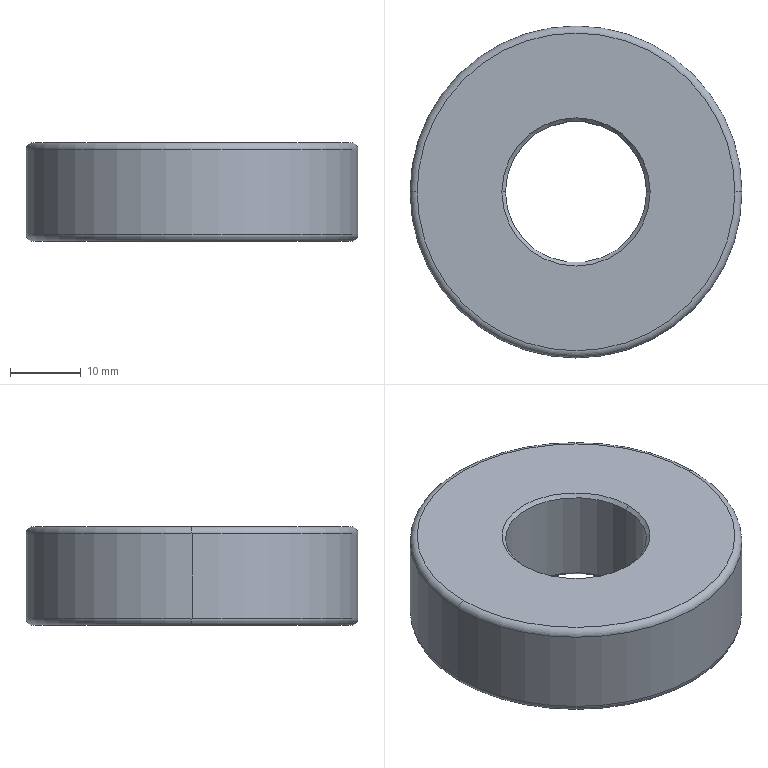Part | SolidWorks | features BaseBody 1 | 1 solid | 14 faces | box 47 x 47 x 14 mm | volume 19812 mm3 | cone 4 | torus 4 | cylinder 4 | plane 2 | commonest cylinder face diameters 20 x2 47 x2
STEP:
#1=CARTESIAN_POINT('',(-10.,0.,13.5));
#2=VERTEX_POINT('',#1);
#3=CARTESIAN_POINT('',(10.,0.,13.5));
#4=VERTEX_POINT('',#3);
#5=CARTESIAN_POINT('',(0.,0.,13.5));
#6=DIRECTION('',(0.,0.,1.));
#7=DIRECTION('',(1.,0.,0.));
#8=AXIS2_PLACEMENT_3D('',#5,#6,#7);
#9=CIRCLE('',#8,10.);
#10=EDGE_CURVE('',#2,#4,#9,.T.);
#11=ORIENTED_EDGE('',*,*,#10,.F.);
#12=CARTESIAN_POINT('',(-10.5,0.,14.));
#13=VERTEX_POINT('',#12);
#14=CARTESIAN_POINT('',(-10.,0.,13.5));
#15=DIRECTION('',(-0.7071,0.,0.7071));
#16=VECTOR('',#15,1000.);
#17=LINE('',#14,#16);
#18=EDGE_CURVE('',#2,#13,#17,.T.);
#19=ORIENTED_EDGE('',*,*,#18,.T.);
#20=CARTESIAN_POINT('',(10.5,0.,14.));
#21=VERTEX_POINT('',#20);
#22=CARTESIAN_POINT('',(0.,0.,14.));
#23=DIRECTION('',(0.,0.,-1.));
#24=DIRECTION('',(1.,0.,0.));
#25=AXIS2_PLACEMENT_3D('',#22,#23,#24);
#26=CIRCLE('',#25,10.5);
#27=EDGE_CURVE('',#21,#13,#26,.T.);
#28=ORIENTED_EDGE('',*,*,#27,.F.);
#29=CARTESIAN_POINT('',(10.,0.,13.5));
#30=DIRECTION('',(0.7071,0.,0.7071));
#31=VECTOR('',#30,1000.);
#32=LINE('',#29,#31);
#33=EDGE_CURVE('',#4,#21,#32,.T.);
#34=ORIENTED_EDGE('',*,*,#33,.F.);
#35=EDGE_LOOP('',(#11,#19,#28,#34));
#36=FACE_OUTER_BOUND('',#35,.T.);
#37=CARTESIAN_POINT('',(0.,0.,13.5));
#38=DIRECTION('',(0.,0.,1.));
#39=DIRECTION('',(1.,0.,0.));
#40=AXIS2_PLACEMENT_3D('',#37,#38,#39);
#41=CONICAL_SURFACE('',#40,10.,0.7854);
#42=ADVANCED_FACE('',(#36),#41,.F.);
#43=CARTESIAN_POINT('',(10.,0.,0.5));
#44=VERTEX_POINT('',#43);
#45=CARTESIAN_POINT('',(-10.,0.,0.5));
#46=VERTEX_POINT('',#45);
#47=CARTESIAN_POINT('',(0.,0.,0.5));
#48=DIRECTION('',(0.,0.,-1.));
#49=DIRECTION('',(1.,0.,0.));
#50=AXIS2_PLACEMENT_3D('',#47,#48,#49);
#51=CIRCLE('',#50,10.);
#52=EDGE_CURVE('',#44,#46,#51,.T.);
#53=ORIENTED_EDGE('',*,*,#52,.F.);
#54=CARTESIAN_POINT('',(10.5,0.,0.));
#55=VERTEX_POINT('',#54);
#56=CARTESIAN_POINT('',(10.5,0.,0.));
#57=DIRECTION('',(0.7071,0.,-0.7071));
#58=VECTOR('',#57,1000.);
#59=LINE('',#56,#58);
#60=EDGE_CURVE('',#44,#55,#59,.T.);
#61=ORIENTED_EDGE('',*,*,#60,.T.);
#62=CARTESIAN_POINT('',(-10.5,0.,0.));
#63=VERTEX_POINT('',#62);
#64=CARTESIAN_POINT('',(0.,0.,0.));
#65=DIRECTION('',(0.,0.,1.));
#66=DIRECTION('',(1.,0.,0.));
#67=AXIS2_PLACEMENT_3D('',#64,#65,#66);
#68=CIRCLE('',#67,10.5);
#69=EDGE_CURVE('',#63,#55,#68,.T.);
#70=ORIENTED_EDGE('',*,*,#69,.F.);
#71=CARTESIAN_POINT('',(-10.5,0.,0.));
#72=DIRECTION('',(-0.7071,0.,-0.7071));
#73=VECTOR('',#72,1000.);
#74=LINE('',#71,#73);
#75=EDGE_CURVE('',#46,#63,#74,.T.);
#76=ORIENTED_EDGE('',*,*,#75,.F.);
#77=EDGE_LOOP('',(#53,#61,#70,#76));
#78=FACE_OUTER_BOUND('',#77,.T.);
#79=CARTESIAN_POINT('',(0.,0.,0.));
#80=DIRECTION('',(0.,0.,-1.));
#81=DIRECTION('',(-1.,0.,0.));
#82=AXIS2_PLACEMENT_3D('',#79,#80,#81);
#83=CONICAL_SURFACE('',#82,10.5,0.7854);
#84=ADVANCED_FACE('',(#78),#83,.F.);
#85=CARTESIAN_POINT('',(-23.5,0.,13.));
#86=VERTEX_POINT('',#85);
#87=CARTESIAN_POINT('',(23.5,0.,13.));
#88=VERTEX_POINT('',#87);
#89=CARTESIAN_POINT('',(0.,0.,13.));
#90=DIRECTION('',(0.,0.,-1.));
#91=DIRECTION('',(1.,0.,0.));
#92=AXIS2_PLACEMENT_3D('',#89,#90,#91);
#93=CIRCLE('',#92,23.5);
#94=EDGE_CURVE('',#86,#88,#93,.T.);
#95=ORIENTED_EDGE('',*,*,#94,.F.);
#96=CARTESIAN_POINT('',(-22.5,0.,14.));
#97=VERTEX_POINT('',#96);
#98=CARTESIAN_POINT('',(-22.5,0.,13.));
#99=DIRECTION('',(0.,1.,0.));
#100=DIRECTION('',(-1.,0.,0.));
#101=AXIS2_PLACEMENT_3D('',#98,#99,#100);
#102=CIRCLE('',#101,1.);
#103=EDGE_CURVE('',#86,#97,#102,.T.);
#104=ORIENTED_EDGE('',*,*,#103,.T.);
#105=CARTESIAN_POINT('',(22.5,0.,14.));
#106=VERTEX_POINT('',#105);
#107=CARTESIAN_POINT('',(0.,0.,14.));
#108=DIRECTION('',(0.,0.,1.));
#109=DIRECTION('',(1.,0.,0.));
#110=AXIS2_PLACEMENT_3D('',#107,#108,#109);
#111=CIRCLE('',#110,22.5);
#112=EDGE_CURVE('',#106,#97,#111,.T.);
#113=ORIENTED_EDGE('',*,*,#112,.F.);
#114=CARTESIAN_POINT('',(22.5,0.,13.));
#115=DIRECTION('',(0.,-1.,0.));
#116=DIRECTION('',(0.,0.,-1.));
#117=AXIS2_PLACEMENT_3D('',#114,#115,#116);
#118=CIRCLE('',#117,1.);
#119=EDGE_CURVE('',#88,#106,#118,.T.);
#120=ORIENTED_EDGE('',*,*,#119,.F.);
#121=EDGE_LOOP('',(#95,#104,#113,#120));
#122=FACE_OUTER_BOUND('',#121,.T.);
#123=CARTESIAN_POINT('',(0.,0.,13.));
#124=DIRECTION('',(0.,0.,1.));
#125=DIRECTION('',(1.,0.,0.));
#126=AXIS2_PLACEMENT_3D('',#123,#124,#125);
#127=TOROIDAL_SURFACE('',#126,22.5,1.);
#128=ADVANCED_FACE('',(#122),#127,.T.);
#129=CARTESIAN_POINT('',(-22.5,0.,0.));
#130=VERTEX_POINT('',#129);
#131=CARTESIAN_POINT('',(22.5,0.,0.));
#132=VERTEX_POINT('',#131);
#133=CARTESIAN_POINT('',(0.,0.,0.));
#134=DIRECTION('',(0.,0.,-1.));
#135=DIRECTION('',(1.,0.,0.));
#136=AXIS2_PLACEMENT_3D('',#133,#134,#135);
#137=CIRCLE('',#136,22.5);
#138=EDGE_CURVE('',#130,#132,#137,.T.);
#139=ORIENTED_EDGE('',*,*,#138,.F.);
#140=CARTESIAN_POINT('',(-23.5,0.,1.));
#141=VERTEX_POINT('',#140);
#142=CARTESIAN_POINT('',(-22.5,0.,1.));
#143=DIRECTION('',(0.,1.,0.));
#144=DIRECTION('',(-1.,0.,0.));
#145=AXIS2_PLACEMENT_3D('',#142,#143,#144);
#146=CIRCLE('',#145,1.);
#147=EDGE_CURVE('',#130,#141,#146,.T.);
#148=ORIENTED_EDGE('',*,*,#147,.T.);
#149=CARTESIAN_POINT('',(23.5,0.,1.));
#150=VERTEX_POINT('',#149);
#151=CARTESIAN_POINT('',(0.,0.,1.));
#152=DIRECTION('',(0.,0.,1.));
#153=DIRECTION('',(1.,0.,0.));
#154=AXIS2_PLACEMENT_3D('',#151,#152,#153);
#155=CIRCLE('',#154,23.5);
#156=EDGE_CURVE('',#150,#141,#155,.T.);
#157=ORIENTED_EDGE('',*,*,#156,.F.);
#158=CARTESIAN_POINT('',(22.5,0.,1.));
#159=DIRECTION('',(0.,-1.,0.));
#160=DIRECTION('',(0.,0.,-1.));
#161=AXIS2_PLACEMENT_3D('',#158,#159,#160);
#162=CIRCLE('',#161,1.);
#163=EDGE_CURVE('',#132,#150,#162,.T.);
#164=ORIENTED_EDGE('',*,*,#163,.F.);
#165=EDGE_LOOP('',(#139,#148,#157,#164));
#166=FACE_OUTER_BOUND('',#165,.T.);
#167=CARTESIAN_POINT('',(0.,0.,1.));
#168=DIRECTION('',(0.,0.,1.));
#169=DIRECTION('',(1.,0.,0.));
#170=AXIS2_PLACEMENT_3D('',#167,#168,#169);
#171=TOROIDAL_SURFACE('',#170,22.5,1.);
#172=ADVANCED_FACE('',(#166),#171,.T.);
#173=ORIENTED_EDGE('',*,*,#10,.T.);
#174=CARTESIAN_POINT('',(10.,0.,14.));
#175=DIRECTION('',(0.,0.,-1.));
#176=VECTOR('',#175,1000.);
#177=LINE('',#174,#176);
#178=EDGE_CURVE('',#4,#44,#177,.T.);
#179=ORIENTED_EDGE('',*,*,#178,.T.);
#180=ORIENTED_EDGE('',*,*,#52,.T.);
#181=CARTESIAN_POINT('',(-10.,0.,14.));
#182=DIRECTION('',(0.,0.,-1.));
#183=VECTOR('',#182,1000.);
#184=LINE('',#181,#183);
#185=EDGE_CURVE('',#2,#46,#184,.T.);
#186=ORIENTED_EDGE('',*,*,#185,.F.);
#187=EDGE_LOOP('',(#173,#179,#180,#186));
#188=FACE_OUTER_BOUND('',#187,.T.);
#189=CARTESIAN_POINT('',(0.,0.,14.));
#190=DIRECTION('',(0.,0.,-1.));
#191=DIRECTION('',(-1.,0.,0.));
#192=AXIS2_PLACEMENT_3D('',#189,#190,#191);
#193=CYLINDRICAL_SURFACE('',#192,10.);
#194=ADVANCED_FACE('',(#188),#193,.F.);
#195=ORIENTED_EDGE('',*,*,#94,.T.);
#196=CARTESIAN_POINT('',(23.5,0.,14.));
#197=DIRECTION('',(0.,0.,-1.));
#198=VECTOR('',#197,1000.);
#199=LINE('',#196,#198);
#200=EDGE_CURVE('',#88,#150,#199,.T.);
#201=ORIENTED_EDGE('',*,*,#200,.T.);
#202=ORIENTED_EDGE('',*,*,#156,.T.);
#203=CARTESIAN_POINT('',(-23.5,0.,14.));
#204=DIRECTION('',(0.,0.,-1.));
#205=VECTOR('',#204,1000.);
#206=LINE('',#203,#205);
#207=EDGE_CURVE('',#86,#141,#206,.T.);
#208=ORIENTED_EDGE('',*,*,#207,.F.);
#209=EDGE_LOOP('',(#195,#201,#202,#208));
#210=FACE_OUTER_BOUND('',#209,.T.);
#211=CARTESIAN_POINT('',(0.,0.,14.));
#212=DIRECTION('',(0.,0.,-1.));
#213=DIRECTION('',(-1.,0.,0.));
#214=AXIS2_PLACEMENT_3D('',#211,#212,#213);
#215=CYLINDRICAL_SURFACE('',#214,23.5);
#216=ADVANCED_FACE('',(#210),#215,.T.);
#217=ORIENTED_EDGE('',*,*,#69,.T.);
#218=CARTESIAN_POINT('',(0.,0.,0.));
#219=DIRECTION('',(0.,0.,1.));
#220=DIRECTION('',(1.,0.,0.));
#221=AXIS2_PLACEMENT_3D('',#218,#219,#220);
#222=CIRCLE('',#221,10.5);
#223=EDGE_CURVE('',#55,#63,#222,.T.);
#224=ORIENTED_EDGE('',*,*,#223,.T.);
#225=EDGE_LOOP('',(#217,#224));
#226=FACE_BOUND('',#225,.T.);
#227=CARTESIAN_POINT('',(0.,0.,0.));
#228=DIRECTION('',(0.,0.,-1.));
#229=DIRECTION('',(1.,0.,0.));
#230=AXIS2_PLACEMENT_3D('',#227,#228,#229);
#231=CIRCLE('',#230,22.5);
#232=EDGE_CURVE('',#132,#130,#231,.T.);
#233=ORIENTED_EDGE('',*,*,#232,.T.);
#234=ORIENTED_EDGE('',*,*,#138,.T.);
#235=EDGE_LOOP('',(#233,#234));
#236=FACE_OUTER_BOUND('',#235,.T.);
#237=CARTESIAN_POINT('',(0.,0.,0.));
#238=DIRECTION('',(0.,0.,1.));
#239=DIRECTION('',(1.,0.,0.));
#240=AXIS2_PLACEMENT_3D('',#237,#238,#239);
#241=PLANE('',#240);
#242=ADVANCED_FACE('',(#226,#236),#241,.F.);
#243=ORIENTED_EDGE('',*,*,#27,.T.);
#244=CARTESIAN_POINT('',(0.,0.,14.));
#245=DIRECTION('',(0.,0.,-1.));
#246=DIRECTION('',(1.,0.,0.));
#247=AXIS2_PLACEMENT_3D('',#244,#245,#246);
#248=CIRCLE('',#247,10.5);
#249=EDGE_CURVE('',#13,#21,#248,.T.);
#250=ORIENTED_EDGE('',*,*,#249,.T.);
#251=EDGE_LOOP('',(#243,#250));
#252=FACE_BOUND('',#251,.T.);
#253=ORIENTED_EDGE('',*,*,#112,.T.);
#254=CARTESIAN_POINT('',(0.,0.,14.));
#255=DIRECTION('',(0.,0.,1.));
#256=DIRECTION('',(1.,0.,0.));
#257=AXIS2_PLACEMENT_3D('',#254,#255,#256);
#258=CIRCLE('',#257,22.5);
#259=EDGE_CURVE('',#97,#106,#258,.T.);
#260=ORIENTED_EDGE('',*,*,#259,.T.);
#261=EDGE_LOOP('',(#253,#260));
#262=FACE_OUTER_BOUND('',#261,.T.);
#263=CARTESIAN_POINT('',(0.,0.,14.));
#264=DIRECTION('',(0.,0.,1.));
#265=DIRECTION('',(1.,0.,0.));
#266=AXIS2_PLACEMENT_3D('',#263,#264,#265);
#267=PLANE('',#266);
#268=ADVANCED_FACE('',(#252,#262),#267,.T.);
#269=ORIENTED_EDGE('',*,*,#200,.F.);
#270=CARTESIAN_POINT('',(0.,0.,13.));
#271=DIRECTION('',(0.,0.,-1.));
#272=DIRECTION('',(1.,0.,0.));
#273=AXIS2_PLACEMENT_3D('',#270,#271,#272);
#274=CIRCLE('',#273,23.5);
#275=EDGE_CURVE('',#88,#86,#274,.T.);
#276=ORIENTED_EDGE('',*,*,#275,.T.);
#277=ORIENTED_EDGE('',*,*,#207,.T.);
#278=CARTESIAN_POINT('',(0.,0.,1.));
#279=DIRECTION('',(0.,0.,1.));
#280=DIRECTION('',(1.,0.,0.));
#281=AXIS2_PLACEMENT_3D('',#278,#279,#280);
#282=CIRCLE('',#281,23.5);
#283=EDGE_CURVE('',#141,#150,#282,.T.);
#284=ORIENTED_EDGE('',*,*,#283,.T.);
#285=EDGE_LOOP('',(#269,#276,#277,#284));
#286=FACE_OUTER_BOUND('',#285,.T.);
#287=CARTESIAN_POINT('',(0.,0.,14.));
#288=DIRECTION('',(0.,0.,-1.));
#289=DIRECTION('',(-1.,0.,0.));
#290=AXIS2_PLACEMENT_3D('',#287,#288,#289);
#291=CYLINDRICAL_SURFACE('',#290,23.5);
#292=ADVANCED_FACE('',(#286),#291,.T.);
#293=ORIENTED_EDGE('',*,*,#178,.F.);
#294=CARTESIAN_POINT('',(0.,0.,13.5));
#295=DIRECTION('',(0.,0.,1.));
#296=DIRECTION('',(1.,0.,0.));
#297=AXIS2_PLACEMENT_3D('',#294,#295,#296);
#298=CIRCLE('',#297,10.);
#299=EDGE_CURVE('',#4,#2,#298,.T.);
#300=ORIENTED_EDGE('',*,*,#299,.T.);
#301=ORIENTED_EDGE('',*,*,#185,.T.);
#302=CARTESIAN_POINT('',(0.,0.,0.5));
#303=DIRECTION('',(0.,0.,-1.));
#304=DIRECTION('',(1.,0.,0.));
#305=AXIS2_PLACEMENT_3D('',#302,#303,#304);
#306=CIRCLE('',#305,10.);
#307=EDGE_CURVE('',#46,#44,#306,.T.);
#308=ORIENTED_EDGE('',*,*,#307,.T.);
#309=EDGE_LOOP('',(#293,#300,#301,#308));
#310=FACE_OUTER_BOUND('',#309,.T.);
#311=CARTESIAN_POINT('',(0.,0.,14.));
#312=DIRECTION('',(0.,0.,-1.));
#313=DIRECTION('',(-1.,0.,0.));
#314=AXIS2_PLACEMENT_3D('',#311,#312,#313);
#315=CYLINDRICAL_SURFACE('',#314,10.);
#316=ADVANCED_FACE('',(#310),#315,.F.);
#317=ORIENTED_EDGE('',*,*,#147,.F.);
#318=ORIENTED_EDGE('',*,*,#232,.F.);
#319=ORIENTED_EDGE('',*,*,#163,.T.);
#320=ORIENTED_EDGE('',*,*,#283,.F.);
#321=EDGE_LOOP('',(#317,#318,#319,#320));
#322=FACE_OUTER_BOUND('',#321,.T.);
#323=CARTESIAN_POINT('',(0.,0.,1.));
#324=DIRECTION('',(0.,0.,1.));
#325=DIRECTION('',(1.,0.,0.));
#326=AXIS2_PLACEMENT_3D('',#323,#324,#325);
#327=TOROIDAL_SURFACE('',#326,22.5,1.);
#328=ADVANCED_FACE('',(#322),#327,.T.);
#329=ORIENTED_EDGE('',*,*,#103,.F.);
#330=ORIENTED_EDGE('',*,*,#275,.F.);
#331=ORIENTED_EDGE('',*,*,#119,.T.);
#332=ORIENTED_EDGE('',*,*,#259,.F.);
#333=EDGE_LOOP('',(#329,#330,#331,#332));
#334=FACE_OUTER_BOUND('',#333,.T.);
#335=CARTESIAN_POINT('',(0.,0.,13.));
#336=DIRECTION('',(0.,0.,1.));
#337=DIRECTION('',(1.,0.,0.));
#338=AXIS2_PLACEMENT_3D('',#335,#336,#337);
#339=TOROIDAL_SURFACE('',#338,22.5,1.);
#340=ADVANCED_FACE('',(#334),#339,.T.);
#341=ORIENTED_EDGE('',*,*,#60,.F.);
#342=ORIENTED_EDGE('',*,*,#307,.F.);
#343=ORIENTED_EDGE('',*,*,#75,.T.);
#344=ORIENTED_EDGE('',*,*,#223,.F.);
#345=EDGE_LOOP('',(#341,#342,#343,#344));
#346=FACE_OUTER_BOUND('',#345,.T.);
#347=CARTESIAN_POINT('',(0.,0.,0.));
#348=DIRECTION('',(0.,0.,-1.));
#349=DIRECTION('',(-1.,0.,0.));
#350=AXIS2_PLACEMENT_3D('',#347,#348,#349);
#351=CONICAL_SURFACE('',#350,10.5,0.7854);
#352=ADVANCED_FACE('',(#346),#351,.F.);
#353=ORIENTED_EDGE('',*,*,#18,.F.);
#354=ORIENTED_EDGE('',*,*,#299,.F.);
#355=ORIENTED_EDGE('',*,*,#33,.T.);
#356=ORIENTED_EDGE('',*,*,#249,.F.);
#357=EDGE_LOOP('',(#353,#354,#355,#356));
#358=FACE_OUTER_BOUND('',#357,.T.);
#359=CARTESIAN_POINT('',(0.,0.,13.5));
#360=DIRECTION('',(0.,0.,1.));
#361=DIRECTION('',(1.,0.,0.));
#362=AXIS2_PLACEMENT_3D('',#359,#360,#361);
#363=CONICAL_SURFACE('',#362,10.,0.7854);
#364=ADVANCED_FACE('',(#358),#363,.F.);
#365=CLOSED_SHELL('',(#42,#84,#128,#172,#194,#216,#242,#268,#292,#316,#328,#340,#352,#364));
#366=MANIFOLD_SOLID_BREP('',#365);
#367=CARTESIAN_POINT('',(0.,0.,0.));
#368=DIRECTION('',(0.,0.,1.));
#369=DIRECTION('',(1.,0.,0.));
#370=AXIS2_PLACEMENT_3D('',#367,#368,#369);
#371=(LENGTH_UNIT()NAMED_UNIT(*)SI_UNIT(.MILLI.,.METRE.));
#372=UNCERTAINTY_MEASURE_WITH_UNIT(LENGTH_MEASURE(0.00001),#371,'','');
#373=(NAMED_UNIT(*)PLANE_ANGLE_UNIT()SI_UNIT($,.RADIAN.));
#374=(NAMED_UNIT(*)SI_UNIT($,.STERADIAN.)SOLID_ANGLE_UNIT());
#375=(GEOMETRIC_REPRESENTATION_CONTEXT(3)GLOBAL_UNCERTAINTY_ASSIGNED_CONTEXT((#372))GLOBAL_UNIT_ASSIGNED_CONTEXT((#371,#373,#374))REPRESENTATION_CONTEXT('',''));
#376=ADVANCED_BREP_SHAPE_REPRESENTATION('',(#366,#370),#375);